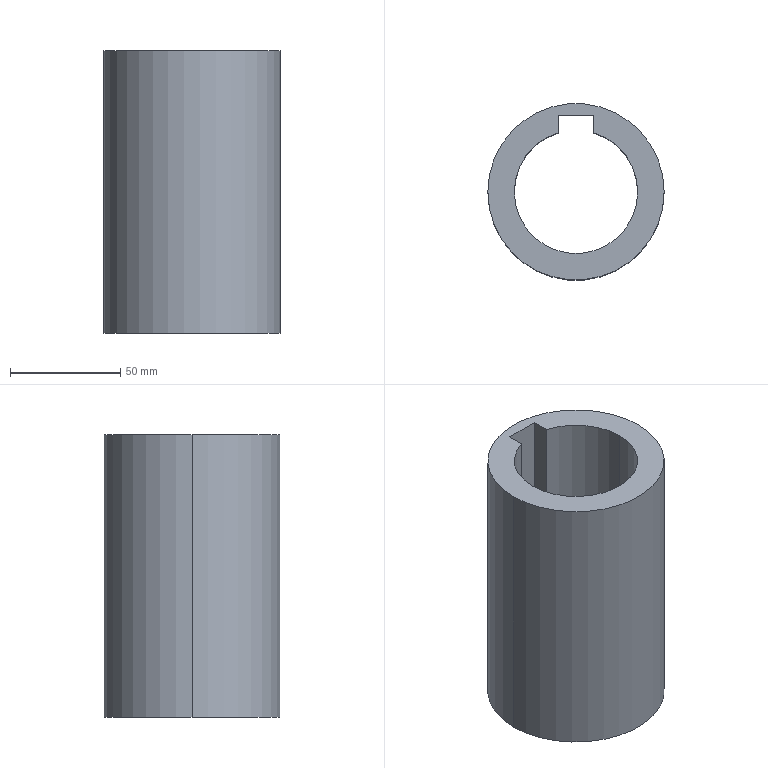Part | SolidWorks | features BaseBody 1 | 1 solid | 10 faces | box 80 x 80 x 128 mm | volume 313826 mm3 | plane 5 | cylinder 5 | commonest cylinder face diameters 56 x3 80 x2
STEP:
#1=CARTESIAN_POINT('',(273.077,980.082,627.507));
#2=VERTEX_POINT('',#1);
#3=CARTESIAN_POINT('',(273.077,987.849,627.507));
#4=VERTEX_POINT('',#3);
#5=CARTESIAN_POINT('',(273.077,987.849,627.507));
#6=DIRECTION('',(0.,1.,0.));
#7=VECTOR('',#6,1000.);
#8=LINE('',#5,#7);
#9=EDGE_CURVE('',#2,#4,#8,.T.);
#10=ORIENTED_EDGE('',*,*,#9,.F.);
#11=CARTESIAN_POINT('',(273.077,980.082,755.507));
#12=VERTEX_POINT('',#11);
#13=CARTESIAN_POINT('',(273.077,980.082,755.507));
#14=DIRECTION('',(0.,0.,-1.));
#15=VECTOR('',#14,1000.);
#16=LINE('',#13,#15);
#17=EDGE_CURVE('',#12,#2,#16,.T.);
#18=ORIENTED_EDGE('',*,*,#17,.F.);
#19=CARTESIAN_POINT('',(273.077,987.849,755.507));
#20=VERTEX_POINT('',#19);
#21=CARTESIAN_POINT('',(273.077,987.849,755.507));
#22=DIRECTION('',(0.,1.,0.));
#23=VECTOR('',#22,1000.);
#24=LINE('',#21,#23);
#25=EDGE_CURVE('',#12,#20,#24,.T.);
#26=ORIENTED_EDGE('',*,*,#25,.T.);
#27=CARTESIAN_POINT('',(273.077,987.849,755.507));
#28=DIRECTION('',(0.,0.,-1.));
#29=VECTOR('',#28,1000.);
#30=LINE('',#27,#29);
#31=EDGE_CURVE('',#20,#4,#30,.T.);
#32=ORIENTED_EDGE('',*,*,#31,.T.);
#33=EDGE_LOOP('',(#10,#18,#26,#32));
#34=FACE_OUTER_BOUND('',#33,.T.);
#35=CARTESIAN_POINT('',(273.077,987.849,755.507));
#36=DIRECTION('',(1.,0.,0.));
#37=DIRECTION('',(0.,1.,0.));
#38=AXIS2_PLACEMENT_3D('',#35,#36,#37);
#39=PLANE('',#38);
#40=ADVANCED_FACE('',(#34),#39,.F.);
#41=CARTESIAN_POINT('',(257.077,987.849,627.507));
#42=VERTEX_POINT('',#41);
#43=CARTESIAN_POINT('',(257.077,987.849,627.507));
#44=DIRECTION('',(-1.,0.,0.));
#45=VECTOR('',#44,1000.);
#46=LINE('',#43,#45);
#47=EDGE_CURVE('',#4,#42,#46,.T.);
#48=ORIENTED_EDGE('',*,*,#47,.F.);
#49=ORIENTED_EDGE('',*,*,#31,.F.);
#50=CARTESIAN_POINT('',(257.077,987.849,755.507));
#51=VERTEX_POINT('',#50);
#52=CARTESIAN_POINT('',(257.077,987.849,755.507));
#53=DIRECTION('',(-1.,0.,0.));
#54=VECTOR('',#53,1000.);
#55=LINE('',#52,#54);
#56=EDGE_CURVE('',#20,#51,#55,.T.);
#57=ORIENTED_EDGE('',*,*,#56,.T.);
#58=CARTESIAN_POINT('',(257.077,987.849,755.507));
#59=DIRECTION('',(0.,0.,-1.));
#60=VECTOR('',#59,1000.);
#61=LINE('',#58,#60);
#62=EDGE_CURVE('',#51,#42,#61,.T.);
#63=ORIENTED_EDGE('',*,*,#62,.T.);
#64=EDGE_LOOP('',(#48,#49,#57,#63));
#65=FACE_OUTER_BOUND('',#64,.T.);
#66=CARTESIAN_POINT('',(257.077,987.849,755.507));
#67=DIRECTION('',(0.,1.,0.));
#68=DIRECTION('',(1.,0.,0.));
#69=AXIS2_PLACEMENT_3D('',#66,#67,#68);
#70=PLANE('',#69);
#71=ADVANCED_FACE('',(#65),#70,.F.);
#72=CARTESIAN_POINT('',(257.077,980.082,627.507));
#73=VERTEX_POINT('',#72);
#74=CARTESIAN_POINT('',(257.077,980.082,627.507));
#75=DIRECTION('',(0.,-1.,0.));
#76=VECTOR('',#75,1000.);
#77=LINE('',#74,#76);
#78=EDGE_CURVE('',#42,#73,#77,.T.);
#79=ORIENTED_EDGE('',*,*,#78,.F.);
#80=ORIENTED_EDGE('',*,*,#62,.F.);
#81=CARTESIAN_POINT('',(257.077,980.082,755.507));
#82=VERTEX_POINT('',#81);
#83=CARTESIAN_POINT('',(257.077,980.082,755.507));
#84=DIRECTION('',(0.,-1.,0.));
#85=VECTOR('',#84,1000.);
#86=LINE('',#83,#85);
#87=EDGE_CURVE('',#51,#82,#86,.T.);
#88=ORIENTED_EDGE('',*,*,#87,.T.);
#89=CARTESIAN_POINT('',(257.077,980.082,755.507));
#90=DIRECTION('',(0.,0.,-1.));
#91=VECTOR('',#90,1000.);
#92=LINE('',#89,#91);
#93=EDGE_CURVE('',#82,#73,#92,.T.);
#94=ORIENTED_EDGE('',*,*,#93,.T.);
#95=EDGE_LOOP('',(#79,#80,#88,#94));
#96=FACE_OUTER_BOUND('',#95,.T.);
#97=CARTESIAN_POINT('',(257.077,980.082,755.507));
#98=DIRECTION('',(-1.,0.,0.));
#99=DIRECTION('',(0.,0.,1.));
#100=AXIS2_PLACEMENT_3D('',#97,#98,#99);
#101=PLANE('',#100);
#102=ADVANCED_FACE('',(#96),#101,.F.);
#103=CARTESIAN_POINT('',(237.077,953.249,755.507));
#104=VERTEX_POINT('',#103);
#105=CARTESIAN_POINT('',(237.077,953.249,627.507));
#106=VERTEX_POINT('',#105);
#107=CARTESIAN_POINT('',(237.077,953.249,755.507));
#108=DIRECTION('',(0.,0.,-1.));
#109=VECTOR('',#108,1000.);
#110=LINE('',#107,#109);
#111=EDGE_CURVE('',#104,#106,#110,.T.);
#112=ORIENTED_EDGE('',*,*,#111,.T.);
#113=CARTESIAN_POINT('',(265.077,953.249,627.507));
#114=DIRECTION('',(0.,0.,1.));
#115=DIRECTION('',(1.,0.,0.));
#116=AXIS2_PLACEMENT_3D('',#113,#114,#115);
#117=CIRCLE('',#116,28.);
#118=EDGE_CURVE('',#73,#106,#117,.T.);
#119=ORIENTED_EDGE('',*,*,#118,.F.);
#120=ORIENTED_EDGE('',*,*,#93,.F.);
#121=CARTESIAN_POINT('',(265.077,953.249,755.507));
#122=DIRECTION('',(0.,0.,1.));
#123=DIRECTION('',(1.,0.,0.));
#124=AXIS2_PLACEMENT_3D('',#121,#122,#123);
#125=CIRCLE('',#124,28.);
#126=EDGE_CURVE('',#82,#104,#125,.T.);
#127=ORIENTED_EDGE('',*,*,#126,.T.);
#128=EDGE_LOOP('',(#112,#119,#120,#127));
#129=FACE_OUTER_BOUND('',#128,.T.);
#130=CARTESIAN_POINT('',(265.077,953.249,755.507));
#131=DIRECTION('',(0.,0.,-1.));
#132=DIRECTION('',(1.,0.,0.));
#133=AXIS2_PLACEMENT_3D('',#130,#131,#132);
#134=CYLINDRICAL_SURFACE('',#133,28.);
#135=ADVANCED_FACE('',(#129),#134,.F.);
#136=ORIENTED_EDGE('',*,*,#118,.T.);
#137=CARTESIAN_POINT('',(293.077,953.249,627.507));
#138=VERTEX_POINT('',#137);
#139=CARTESIAN_POINT('',(265.077,953.249,627.507));
#140=DIRECTION('',(0.,0.,1.));
#141=DIRECTION('',(1.,0.,0.));
#142=AXIS2_PLACEMENT_3D('',#139,#140,#141);
#143=CIRCLE('',#142,28.);
#144=EDGE_CURVE('',#106,#138,#143,.T.);
#145=ORIENTED_EDGE('',*,*,#144,.T.);
#146=CARTESIAN_POINT('',(265.077,953.249,627.507));
#147=DIRECTION('',(0.,0.,1.));
#148=DIRECTION('',(1.,0.,0.));
#149=AXIS2_PLACEMENT_3D('',#146,#147,#148);
#150=CIRCLE('',#149,28.);
#151=EDGE_CURVE('',#138,#2,#150,.T.);
#152=ORIENTED_EDGE('',*,*,#151,.T.);
#153=ORIENTED_EDGE('',*,*,#9,.T.);
#154=ORIENTED_EDGE('',*,*,#47,.T.);
#155=ORIENTED_EDGE('',*,*,#78,.T.);
#156=EDGE_LOOP('',(#136,#145,#152,#153,#154,#155));
#157=FACE_BOUND('',#156,.T.);
#158=CARTESIAN_POINT('',(305.077,953.249,627.507));
#159=VERTEX_POINT('',#158);
#160=CARTESIAN_POINT('',(225.077,953.249,627.507));
#161=VERTEX_POINT('',#160);
#162=CARTESIAN_POINT('',(265.077,953.249,627.507));
#163=DIRECTION('',(0.,0.,1.));
#164=DIRECTION('',(1.,0.,0.));
#165=AXIS2_PLACEMENT_3D('',#162,#163,#164);
#166=CIRCLE('',#165,40.);
#167=EDGE_CURVE('',#159,#161,#166,.T.);
#168=ORIENTED_EDGE('',*,*,#167,.F.);
#169=CARTESIAN_POINT('',(265.077,953.249,627.507));
#170=DIRECTION('',(0.,0.,1.));
#171=DIRECTION('',(1.,0.,0.));
#172=AXIS2_PLACEMENT_3D('',#169,#170,#171);
#173=CIRCLE('',#172,40.);
#174=EDGE_CURVE('',#161,#159,#173,.T.);
#175=ORIENTED_EDGE('',*,*,#174,.F.);
#176=EDGE_LOOP('',(#168,#175));
#177=FACE_OUTER_BOUND('',#176,.T.);
#178=CARTESIAN_POINT('',(265.077,953.249,627.507));
#179=DIRECTION('',(0.,0.,-1.));
#180=DIRECTION('',(0.,-1.,0.));
#181=AXIS2_PLACEMENT_3D('',#178,#179,#180);
#182=PLANE('',#181);
#183=ADVANCED_FACE('',(#157,#177),#182,.T.);
#184=ORIENTED_EDGE('',*,*,#87,.F.);
#185=ORIENTED_EDGE('',*,*,#56,.F.);
#186=ORIENTED_EDGE('',*,*,#25,.F.);
#187=CARTESIAN_POINT('',(293.077,953.249,755.507));
#188=VERTEX_POINT('',#187);
#189=CARTESIAN_POINT('',(265.077,953.249,755.507));
#190=DIRECTION('',(0.,0.,1.));
#191=DIRECTION('',(1.,0.,0.));
#192=AXIS2_PLACEMENT_3D('',#189,#190,#191);
#193=CIRCLE('',#192,28.);
#194=EDGE_CURVE('',#188,#12,#193,.T.);
#195=ORIENTED_EDGE('',*,*,#194,.F.);
#196=CARTESIAN_POINT('',(265.077,953.249,755.507));
#197=DIRECTION('',(0.,0.,1.));
#198=DIRECTION('',(1.,0.,0.));
#199=AXIS2_PLACEMENT_3D('',#196,#197,#198);
#200=CIRCLE('',#199,28.);
#201=EDGE_CURVE('',#104,#188,#200,.T.);
#202=ORIENTED_EDGE('',*,*,#201,.F.);
#203=ORIENTED_EDGE('',*,*,#126,.F.);
#204=EDGE_LOOP('',(#184,#185,#186,#195,#202,#203));
#205=FACE_BOUND('',#204,.T.);
#206=CARTESIAN_POINT('',(305.077,953.249,755.507));
#207=VERTEX_POINT('',#206);
#208=CARTESIAN_POINT('',(225.077,953.249,755.507));
#209=VERTEX_POINT('',#208);
#210=CARTESIAN_POINT('',(265.077,953.249,755.507));
#211=DIRECTION('',(0.,0.,1.));
#212=DIRECTION('',(1.,0.,0.));
#213=AXIS2_PLACEMENT_3D('',#210,#211,#212);
#214=CIRCLE('',#213,40.);
#215=EDGE_CURVE('',#207,#209,#214,.T.);
#216=ORIENTED_EDGE('',*,*,#215,.T.);
#217=CARTESIAN_POINT('',(265.077,953.249,755.507));
#218=DIRECTION('',(0.,0.,1.));
#219=DIRECTION('',(1.,0.,0.));
#220=AXIS2_PLACEMENT_3D('',#217,#218,#219);
#221=CIRCLE('',#220,40.);
#222=EDGE_CURVE('',#209,#207,#221,.T.);
#223=ORIENTED_EDGE('',*,*,#222,.T.);
#224=EDGE_LOOP('',(#216,#223));
#225=FACE_OUTER_BOUND('',#224,.T.);
#226=CARTESIAN_POINT('',(265.077,953.249,755.507));
#227=DIRECTION('',(0.,0.,-1.));
#228=DIRECTION('',(0.,-1.,0.));
#229=AXIS2_PLACEMENT_3D('',#226,#227,#228);
#230=PLANE('',#229);
#231=ADVANCED_FACE('',(#205,#225),#230,.F.);
#232=CARTESIAN_POINT('',(225.077,953.249,755.507));
#233=DIRECTION('',(0.,0.,-1.));
#234=VECTOR('',#233,1000.);
#235=LINE('',#232,#234);
#236=EDGE_CURVE('',#209,#161,#235,.T.);
#237=ORIENTED_EDGE('',*,*,#236,.T.);
#238=ORIENTED_EDGE('',*,*,#174,.T.);
#239=CARTESIAN_POINT('',(305.077,953.249,755.507));
#240=DIRECTION('',(0.,0.,-1.));
#241=VECTOR('',#240,1000.);
#242=LINE('',#239,#241);
#243=EDGE_CURVE('',#207,#159,#242,.T.);
#244=ORIENTED_EDGE('',*,*,#243,.F.);
#245=ORIENTED_EDGE('',*,*,#222,.F.);
#246=EDGE_LOOP('',(#237,#238,#244,#245));
#247=FACE_OUTER_BOUND('',#246,.T.);
#248=CARTESIAN_POINT('',(265.077,953.249,755.507));
#249=DIRECTION('',(0.,0.,-1.));
#250=DIRECTION('',(1.,0.,0.));
#251=AXIS2_PLACEMENT_3D('',#248,#249,#250);
#252=CYLINDRICAL_SURFACE('',#251,40.);
#253=ADVANCED_FACE('',(#247),#252,.T.);
#254=ORIENTED_EDGE('',*,*,#215,.F.);
#255=ORIENTED_EDGE('',*,*,#243,.T.);
#256=ORIENTED_EDGE('',*,*,#167,.T.);
#257=ORIENTED_EDGE('',*,*,#236,.F.);
#258=EDGE_LOOP('',(#254,#255,#256,#257));
#259=FACE_OUTER_BOUND('',#258,.T.);
#260=CARTESIAN_POINT('',(265.077,953.249,755.507));
#261=DIRECTION('',(0.,0.,-1.));
#262=DIRECTION('',(1.,0.,0.));
#263=AXIS2_PLACEMENT_3D('',#260,#261,#262);
#264=CYLINDRICAL_SURFACE('',#263,40.);
#265=ADVANCED_FACE('',(#259),#264,.T.);
#266=ORIENTED_EDGE('',*,*,#194,.T.);
#267=ORIENTED_EDGE('',*,*,#17,.T.);
#268=ORIENTED_EDGE('',*,*,#151,.F.);
#269=CARTESIAN_POINT('',(293.077,953.249,755.507));
#270=DIRECTION('',(0.,0.,-1.));
#271=VECTOR('',#270,1000.);
#272=LINE('',#269,#271);
#273=EDGE_CURVE('',#188,#138,#272,.T.);
#274=ORIENTED_EDGE('',*,*,#273,.F.);
#275=EDGE_LOOP('',(#266,#267,#268,#274));
#276=FACE_OUTER_BOUND('',#275,.T.);
#277=CARTESIAN_POINT('',(265.077,953.249,755.507));
#278=DIRECTION('',(0.,0.,-1.));
#279=DIRECTION('',(1.,0.,0.));
#280=AXIS2_PLACEMENT_3D('',#277,#278,#279);
#281=CYLINDRICAL_SURFACE('',#280,28.);
#282=ADVANCED_FACE('',(#276),#281,.F.);
#283=ORIENTED_EDGE('',*,*,#201,.T.);
#284=ORIENTED_EDGE('',*,*,#273,.T.);
#285=ORIENTED_EDGE('',*,*,#144,.F.);
#286=ORIENTED_EDGE('',*,*,#111,.F.);
#287=EDGE_LOOP('',(#283,#284,#285,#286));
#288=FACE_OUTER_BOUND('',#287,.T.);
#289=CARTESIAN_POINT('',(265.077,953.249,755.507));
#290=DIRECTION('',(0.,0.,-1.));
#291=DIRECTION('',(1.,0.,0.));
#292=AXIS2_PLACEMENT_3D('',#289,#290,#291);
#293=CYLINDRICAL_SURFACE('',#292,28.);
#294=ADVANCED_FACE('',(#288),#293,.F.);
#295=CLOSED_SHELL('',(#40,#71,#102,#135,#183,#231,#253,#265,#282,#294));
#296=MANIFOLD_SOLID_BREP('',#295);
#297=CARTESIAN_POINT('',(0.,0.,0.));
#298=DIRECTION('',(0.,0.,1.));
#299=DIRECTION('',(1.,0.,0.));
#300=AXIS2_PLACEMENT_3D('',#297,#298,#299);
#301=(LENGTH_UNIT()NAMED_UNIT(*)SI_UNIT(.MILLI.,.METRE.));
#302=UNCERTAINTY_MEASURE_WITH_UNIT(LENGTH_MEASURE(0.00001),#301,'','');
#303=(NAMED_UNIT(*)PLANE_ANGLE_UNIT()SI_UNIT($,.RADIAN.));
#304=(NAMED_UNIT(*)SI_UNIT($,.STERADIAN.)SOLID_ANGLE_UNIT());
#305=(GEOMETRIC_REPRESENTATION_CONTEXT(3)GLOBAL_UNCERTAINTY_ASSIGNED_CONTEXT((#302))GLOBAL_UNIT_ASSIGNED_CONTEXT((#301,#303,#304))REPRESENTATION_CONTEXT('',''));
#306=ADVANCED_BREP_SHAPE_REPRESENTATION('',(#296,#300),#305);